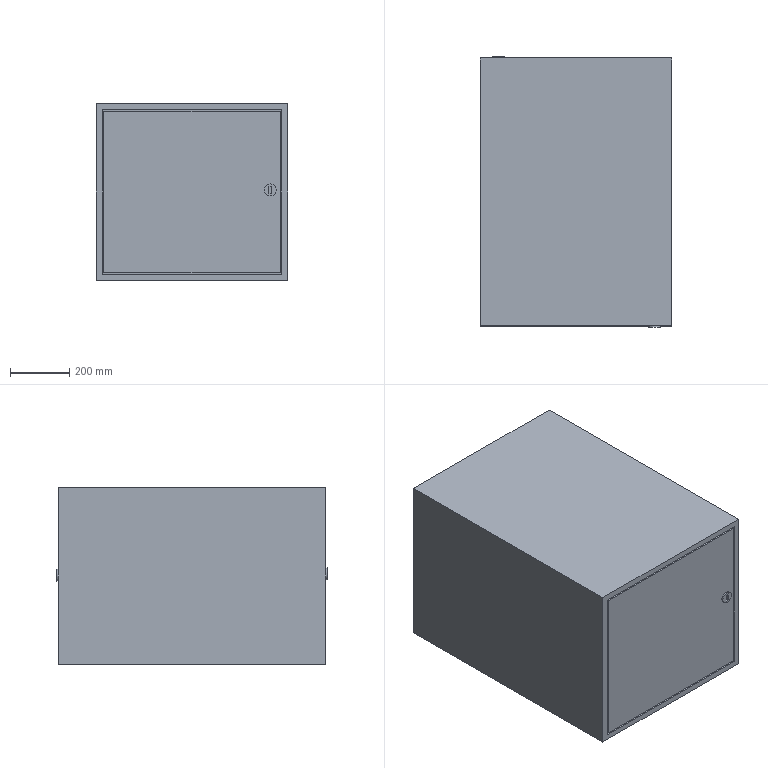Part | SolidWorks | features ICE 6, Extrusion 1 | 1 solid | 42 faces | box 645 x 910 x 594.5 mm | volume 344886947 mm3 | plane 38 | cylinder 4 | commonest cylinder face diameters 40 x4
STEP:
#1=CARTESIAN_POINT('',(-261.326,455.,320.206));
#2=VERTEX_POINT('',#1);
#3=CARTESIAN_POINT('',(-261.326,455.,280.206));
#4=VERTEX_POINT('',#3);
#5=CARTESIAN_POINT('',(-261.326,455.,300.206));
#6=DIRECTION('',(0.,1.,0.));
#7=DIRECTION('',(0.,0.,1.));
#8=AXIS2_PLACEMENT_3D('',#5,#6,#7);
#9=CIRCLE('',#8,20.);
#10=EDGE_CURVE('',#2,#4,#9,.T.);
#11=ORIENTED_EDGE('',*,*,#10,.F.);
#12=CARTESIAN_POINT('',(-261.326,450.,320.206));
#13=VERTEX_POINT('',#12);
#14=CARTESIAN_POINT('',(-261.326,455.,320.206));
#15=DIRECTION('',(0.,-1.,0.));
#16=VECTOR('',#15,1000.);
#17=LINE('',#14,#16);
#18=EDGE_CURVE('',#2,#13,#17,.T.);
#19=ORIENTED_EDGE('',*,*,#18,.T.);
#20=CARTESIAN_POINT('',(-261.326,450.,280.206));
#21=VERTEX_POINT('',#20);
#22=CARTESIAN_POINT('',(-261.326,450.,300.206));
#23=DIRECTION('',(0.,1.,0.));
#24=DIRECTION('',(0.,0.,-1.));
#25=AXIS2_PLACEMENT_3D('',#22,#23,#24);
#26=CIRCLE('',#25,20.);
#27=EDGE_CURVE('',#13,#21,#26,.T.);
#28=ORIENTED_EDGE('',*,*,#27,.T.);
#29=CARTESIAN_POINT('',(-261.326,455.,280.206));
#30=DIRECTION('',(0.,-1.,0.));
#31=VECTOR('',#30,1000.);
#32=LINE('',#29,#31);
#33=EDGE_CURVE('',#4,#21,#32,.T.);
#34=ORIENTED_EDGE('',*,*,#33,.F.);
#35=EDGE_LOOP('',(#11,#19,#28,#34));
#36=FACE_OUTER_BOUND('',#35,.T.);
#37=CARTESIAN_POINT('',(-261.326,455.,300.206));
#38=DIRECTION('',(0.,-1.,0.));
#39=DIRECTION('',(0.,0.,-1.));
#40=AXIS2_PLACEMENT_3D('',#37,#38,#39);
#41=CYLINDRICAL_SURFACE('',#40,20.);
#42=ADVANCED_FACE('',(#36),#41,.T.);
#43=CARTESIAN_POINT('',(263.592,-455.,284.23));
#44=VERTEX_POINT('',#43);
#45=CARTESIAN_POINT('',(263.592,-455.,324.23));
#46=VERTEX_POINT('',#45);
#47=CARTESIAN_POINT('',(263.592,-455.,304.23));
#48=DIRECTION('',(0.,-1.,0.));
#49=DIRECTION('',(0.,0.,-1.));
#50=AXIS2_PLACEMENT_3D('',#47,#48,#49);
#51=CIRCLE('',#50,20.);
#52=EDGE_CURVE('',#44,#46,#51,.T.);
#53=ORIENTED_EDGE('',*,*,#52,.F.);
#54=CARTESIAN_POINT('',(263.592,-450.,284.23));
#55=VERTEX_POINT('',#54);
#56=CARTESIAN_POINT('',(263.592,-455.,284.23));
#57=DIRECTION('',(0.,1.,0.));
#58=VECTOR('',#57,1000.);
#59=LINE('',#56,#58);
#60=EDGE_CURVE('',#44,#55,#59,.T.);
#61=ORIENTED_EDGE('',*,*,#60,.T.);
#62=CARTESIAN_POINT('',(263.592,-450.,324.23));
#63=VERTEX_POINT('',#62);
#64=CARTESIAN_POINT('',(263.592,-450.,304.23));
#65=DIRECTION('',(0.,-1.,0.));
#66=DIRECTION('',(0.,0.,1.));
#67=AXIS2_PLACEMENT_3D('',#64,#65,#66);
#68=CIRCLE('',#67,20.);
#69=EDGE_CURVE('',#55,#63,#68,.T.);
#70=ORIENTED_EDGE('',*,*,#69,.T.);
#71=CARTESIAN_POINT('',(263.592,-455.,324.23));
#72=DIRECTION('',(0.,1.,0.));
#73=VECTOR('',#72,1000.);
#74=LINE('',#71,#73);
#75=EDGE_CURVE('',#46,#63,#74,.T.);
#76=ORIENTED_EDGE('',*,*,#75,.F.);
#77=EDGE_LOOP('',(#53,#61,#70,#76));
#78=FACE_OUTER_BOUND('',#77,.T.);
#79=CARTESIAN_POINT('',(263.592,-455.,304.23));
#80=DIRECTION('',(0.,1.,0.));
#81=DIRECTION('',(0.,0.,1.));
#82=AXIS2_PLACEMENT_3D('',#79,#80,#81);
#83=CYLINDRICAL_SURFACE('',#82,20.);
#84=ADVANCED_FACE('',(#78),#83,.T.);
#85=CARTESIAN_POINT('',(322.5,-450.,0.));
#86=VERTEX_POINT('',#85);
#87=CARTESIAN_POINT('',(322.5,450.,0.));
#88=VERTEX_POINT('',#87);
#89=CARTESIAN_POINT('',(322.5,450.,0.));
#90=DIRECTION('',(0.,1.,0.));
#91=VECTOR('',#90,1000.);
#92=LINE('',#89,#91);
#93=EDGE_CURVE('',#86,#88,#92,.T.);
#94=ORIENTED_EDGE('',*,*,#93,.T.);
#95=CARTESIAN_POINT('',(322.5,450.,594.5));
#96=VERTEX_POINT('',#95);
#97=CARTESIAN_POINT('',(322.5,450.,594.5));
#98=DIRECTION('',(0.,0.,-1.));
#99=VECTOR('',#98,1000.);
#100=LINE('',#97,#99);
#101=EDGE_CURVE('',#96,#88,#100,.T.);
#102=ORIENTED_EDGE('',*,*,#101,.F.);
#103=CARTESIAN_POINT('',(322.5,-450.,594.5));
#104=VERTEX_POINT('',#103);
#105=CARTESIAN_POINT('',(322.5,450.,594.5));
#106=DIRECTION('',(0.,1.,0.));
#107=VECTOR('',#106,1000.);
#108=LINE('',#105,#107);
#109=EDGE_CURVE('',#104,#96,#108,.T.);
#110=ORIENTED_EDGE('',*,*,#109,.F.);
#111=CARTESIAN_POINT('',(322.5,-450.,594.5));
#112=DIRECTION('',(0.,0.,-1.));
#113=VECTOR('',#112,1000.);
#114=LINE('',#111,#113);
#115=EDGE_CURVE('',#104,#86,#114,.T.);
#116=ORIENTED_EDGE('',*,*,#115,.T.);
#117=EDGE_LOOP('',(#94,#102,#110,#116));
#118=FACE_OUTER_BOUND('',#117,.T.);
#119=CARTESIAN_POINT('',(322.5,450.,594.5));
#120=DIRECTION('',(-1.,0.,0.));
#121=DIRECTION('',(0.,-1.,0.));
#122=AXIS2_PLACEMENT_3D('',#119,#120,#121);
#123=PLANE('',#122);
#124=ADVANCED_FACE('',(#118),#123,.F.);
#125=CARTESIAN_POINT('',(-302.5,450.,574.5));
#126=VERTEX_POINT('',#125);
#127=CARTESIAN_POINT('',(302.5,450.,574.5));
#128=VERTEX_POINT('',#127);
#129=CARTESIAN_POINT('',(-302.5,450.,574.5));
#130=DIRECTION('',(1.,0.,0.));
#131=VECTOR('',#130,1000.);
#132=LINE('',#129,#131);
#133=EDGE_CURVE('',#126,#128,#132,.T.);
#134=ORIENTED_EDGE('',*,*,#133,.F.);
#135=CARTESIAN_POINT('',(-302.5,450.,20.));
#136=VERTEX_POINT('',#135);
#137=CARTESIAN_POINT('',(-302.5,450.,20.));
#138=DIRECTION('',(0.,0.,1.));
#139=VECTOR('',#138,1000.);
#140=LINE('',#137,#139);
#141=EDGE_CURVE('',#136,#126,#140,.T.);
#142=ORIENTED_EDGE('',*,*,#141,.F.);
#143=CARTESIAN_POINT('',(302.5,450.,20.));
#144=VERTEX_POINT('',#143);
#145=CARTESIAN_POINT('',(302.5,450.,20.));
#146=DIRECTION('',(-1.,0.,0.));
#147=VECTOR('',#146,1000.);
#148=LINE('',#145,#147);
#149=EDGE_CURVE('',#144,#136,#148,.T.);
#150=ORIENTED_EDGE('',*,*,#149,.F.);
#151=CARTESIAN_POINT('',(302.5,450.,574.5));
#152=DIRECTION('',(0.,0.,-1.));
#153=VECTOR('',#152,1000.);
#154=LINE('',#151,#153);
#155=EDGE_CURVE('',#128,#144,#154,.T.);
#156=ORIENTED_EDGE('',*,*,#155,.F.);
#157=EDGE_LOOP('',(#134,#142,#150,#156));
#158=FACE_BOUND('',#157,.T.);
#159=CARTESIAN_POINT('',(-322.5,450.,0.));
#160=VERTEX_POINT('',#159);
#161=CARTESIAN_POINT('',(-322.5,450.,0.));
#162=DIRECTION('',(-1.,0.,0.));
#163=VECTOR('',#162,1000.);
#164=LINE('',#161,#163);
#165=EDGE_CURVE('',#88,#160,#164,.T.);
#166=ORIENTED_EDGE('',*,*,#165,.T.);
#167=CARTESIAN_POINT('',(-322.5,450.,594.5));
#168=VERTEX_POINT('',#167);
#169=CARTESIAN_POINT('',(-322.5,450.,594.5));
#170=DIRECTION('',(0.,0.,-1.));
#171=VECTOR('',#170,1000.);
#172=LINE('',#169,#171);
#173=EDGE_CURVE('',#168,#160,#172,.T.);
#174=ORIENTED_EDGE('',*,*,#173,.F.);
#175=CARTESIAN_POINT('',(-322.5,450.,594.5));
#176=DIRECTION('',(-1.,0.,0.));
#177=VECTOR('',#176,1000.);
#178=LINE('',#175,#177);
#179=EDGE_CURVE('',#96,#168,#178,.T.);
#180=ORIENTED_EDGE('',*,*,#179,.F.);
#181=ORIENTED_EDGE('',*,*,#101,.T.);
#182=EDGE_LOOP('',(#166,#174,#180,#181));
#183=FACE_OUTER_BOUND('',#182,.T.);
#184=CARTESIAN_POINT('',(-322.5,450.,594.5));
#185=DIRECTION('',(0.,-1.,0.));
#186=DIRECTION('',(0.,0.,-1.));
#187=AXIS2_PLACEMENT_3D('',#184,#185,#186);
#188=PLANE('',#187);
#189=ADVANCED_FACE('',(#158,#183),#188,.F.);
#190=CARTESIAN_POINT('',(-322.5,-450.,0.));
#191=VERTEX_POINT('',#190);
#192=CARTESIAN_POINT('',(-322.5,450.,0.));
#193=DIRECTION('',(0.,-1.,0.));
#194=VECTOR('',#193,1000.);
#195=LINE('',#192,#194);
#196=EDGE_CURVE('',#160,#191,#195,.T.);
#197=ORIENTED_EDGE('',*,*,#196,.T.);
#198=CARTESIAN_POINT('',(-322.5,-450.,594.5));
#199=VERTEX_POINT('',#198);
#200=CARTESIAN_POINT('',(-322.5,-450.,594.5));
#201=DIRECTION('',(0.,0.,-1.));
#202=VECTOR('',#201,1000.);
#203=LINE('',#200,#202);
#204=EDGE_CURVE('',#199,#191,#203,.T.);
#205=ORIENTED_EDGE('',*,*,#204,.F.);
#206=CARTESIAN_POINT('',(-322.5,450.,594.5));
#207=DIRECTION('',(0.,-1.,0.));
#208=VECTOR('',#207,1000.);
#209=LINE('',#206,#208);
#210=EDGE_CURVE('',#168,#199,#209,.T.);
#211=ORIENTED_EDGE('',*,*,#210,.F.);
#212=ORIENTED_EDGE('',*,*,#173,.T.);
#213=EDGE_LOOP('',(#197,#205,#211,#212));
#214=FACE_OUTER_BOUND('',#213,.T.);
#215=CARTESIAN_POINT('',(-322.5,450.,594.5));
#216=DIRECTION('',(1.,0.,0.));
#217=DIRECTION('',(0.,1.,0.));
#218=AXIS2_PLACEMENT_3D('',#215,#216,#217);
#219=PLANE('',#218);
#220=ADVANCED_FACE('',(#214),#219,.F.);
#221=CARTESIAN_POINT('',(302.5,-450.,574.5));
#222=VERTEX_POINT('',#221);
#223=CARTESIAN_POINT('',(-302.5,-450.,574.5));
#224=VERTEX_POINT('',#223);
#225=CARTESIAN_POINT('',(-302.5,-450.,574.5));
#226=DIRECTION('',(-1.,0.,0.));
#227=VECTOR('',#226,1000.);
#228=LINE('',#225,#227);
#229=EDGE_CURVE('',#222,#224,#228,.T.);
#230=ORIENTED_EDGE('',*,*,#229,.F.);
#231=CARTESIAN_POINT('',(302.5,-450.,20.));
#232=VERTEX_POINT('',#231);
#233=CARTESIAN_POINT('',(302.5,-450.,574.5));
#234=DIRECTION('',(0.,0.,1.));
#235=VECTOR('',#234,1000.);
#236=LINE('',#233,#235);
#237=EDGE_CURVE('',#232,#222,#236,.T.);
#238=ORIENTED_EDGE('',*,*,#237,.F.);
#239=CARTESIAN_POINT('',(-302.5,-450.,20.));
#240=VERTEX_POINT('',#239);
#241=CARTESIAN_POINT('',(-302.5,-450.,20.));
#242=DIRECTION('',(1.,0.,0.));
#243=VECTOR('',#242,1000.);
#244=LINE('',#241,#243);
#245=EDGE_CURVE('',#240,#232,#244,.T.);
#246=ORIENTED_EDGE('',*,*,#245,.F.);
#247=CARTESIAN_POINT('',(-302.5,-450.,574.5));
#248=DIRECTION('',(0.,0.,-1.));
#249=VECTOR('',#248,1000.);
#250=LINE('',#247,#249);
#251=EDGE_CURVE('',#224,#240,#250,.T.);
#252=ORIENTED_EDGE('',*,*,#251,.F.);
#253=EDGE_LOOP('',(#230,#238,#246,#252));
#254=FACE_BOUND('',#253,.T.);
#255=CARTESIAN_POINT('',(-322.5,-450.,0.));
#256=DIRECTION('',(1.,0.,0.));
#257=VECTOR('',#256,1000.);
#258=LINE('',#255,#257);
#259=EDGE_CURVE('',#191,#86,#258,.T.);
#260=ORIENTED_EDGE('',*,*,#259,.T.);
#261=ORIENTED_EDGE('',*,*,#115,.F.);
#262=CARTESIAN_POINT('',(-322.5,-450.,594.5));
#263=DIRECTION('',(1.,0.,0.));
#264=VECTOR('',#263,1000.);
#265=LINE('',#262,#264);
#266=EDGE_CURVE('',#199,#104,#265,.T.);
#267=ORIENTED_EDGE('',*,*,#266,.F.);
#268=ORIENTED_EDGE('',*,*,#204,.T.);
#269=EDGE_LOOP('',(#260,#261,#267,#268));
#270=FACE_OUTER_BOUND('',#269,.T.);
#271=CARTESIAN_POINT('',(-322.5,-450.,594.5));
#272=DIRECTION('',(0.,1.,0.));
#273=DIRECTION('',(0.,0.,1.));
#274=AXIS2_PLACEMENT_3D('',#271,#272,#273);
#275=PLANE('',#274);
#276=ADVANCED_FACE('',(#254,#270),#275,.F.);
#277=ORIENTED_EDGE('',*,*,#109,.T.);
#278=ORIENTED_EDGE('',*,*,#179,.T.);
#279=ORIENTED_EDGE('',*,*,#210,.T.);
#280=ORIENTED_EDGE('',*,*,#266,.T.);
#281=EDGE_LOOP('',(#277,#278,#279,#280));
#282=FACE_OUTER_BOUND('',#281,.T.);
#283=CARTESIAN_POINT('',(0.,0.,594.5));
#284=DIRECTION('',(0.,0.,1.));
#285=DIRECTION('',(1.,0.,0.));
#286=AXIS2_PLACEMENT_3D('',#283,#284,#285);
#287=PLANE('',#286);
#288=ADVANCED_FACE('',(#282),#287,.T.);
#289=ORIENTED_EDGE('',*,*,#93,.F.);
#290=ORIENTED_EDGE('',*,*,#259,.F.);
#291=ORIENTED_EDGE('',*,*,#196,.F.);
#292=ORIENTED_EDGE('',*,*,#165,.F.);
#293=EDGE_LOOP('',(#289,#290,#291,#292));
#294=FACE_OUTER_BOUND('',#293,.T.);
#295=CARTESIAN_POINT('',(0.,0.,0.));
#296=DIRECTION('',(0.,0.,1.));
#297=DIRECTION('',(1.,0.,0.));
#298=AXIS2_PLACEMENT_3D('',#295,#296,#297);
#299=PLANE('',#298);
#300=ADVANCED_FACE('',(#294),#299,.F.);
#301=ORIENTED_EDGE('',*,*,#237,.T.);
#302=CARTESIAN_POINT('',(302.5,-440.,574.5));
#303=VERTEX_POINT('',#302);
#304=CARTESIAN_POINT('',(302.5,-440.,574.5));
#305=DIRECTION('',(0.,-1.,0.));
#306=VECTOR('',#305,1000.);
#307=LINE('',#304,#306);
#308=EDGE_CURVE('',#303,#222,#307,.T.);
#309=ORIENTED_EDGE('',*,*,#308,.F.);
#310=CARTESIAN_POINT('',(302.5,-440.,20.));
#311=VERTEX_POINT('',#310);
#312=CARTESIAN_POINT('',(302.5,-440.,574.5));
#313=DIRECTION('',(0.,0.,1.));
#314=VECTOR('',#313,1000.);
#315=LINE('',#312,#314);
#316=EDGE_CURVE('',#311,#303,#315,.T.);
#317=ORIENTED_EDGE('',*,*,#316,.F.);
#318=CARTESIAN_POINT('',(302.5,-440.,20.));
#319=DIRECTION('',(0.,-1.,0.));
#320=VECTOR('',#319,1000.);
#321=LINE('',#318,#320);
#322=EDGE_CURVE('',#311,#232,#321,.T.);
#323=ORIENTED_EDGE('',*,*,#322,.T.);
#324=EDGE_LOOP('',(#301,#309,#317,#323));
#325=FACE_OUTER_BOUND('',#324,.T.);
#326=CARTESIAN_POINT('',(302.5,-440.,574.5));
#327=DIRECTION('',(1.,0.,0.));
#328=DIRECTION('',(0.,0.,-1.));
#329=AXIS2_PLACEMENT_3D('',#326,#327,#328);
#330=PLANE('',#329);
#331=ADVANCED_FACE('',(#325),#330,.F.);
#332=ORIENTED_EDGE('',*,*,#245,.T.);
#333=ORIENTED_EDGE('',*,*,#322,.F.);
#334=CARTESIAN_POINT('',(-302.5,-440.,20.));
#335=VERTEX_POINT('',#334);
#336=CARTESIAN_POINT('',(-302.5,-440.,20.));
#337=DIRECTION('',(1.,0.,0.));
#338=VECTOR('',#337,1000.);
#339=LINE('',#336,#338);
#340=EDGE_CURVE('',#335,#311,#339,.T.);
#341=ORIENTED_EDGE('',*,*,#340,.F.);
#342=CARTESIAN_POINT('',(-302.5,-440.,20.));
#343=DIRECTION('',(0.,-1.,0.));
#344=VECTOR('',#343,1000.);
#345=LINE('',#342,#344);
#346=EDGE_CURVE('',#335,#240,#345,.T.);
#347=ORIENTED_EDGE('',*,*,#346,.T.);
#348=EDGE_LOOP('',(#332,#333,#341,#347));
#349=FACE_OUTER_BOUND('',#348,.T.);
#350=CARTESIAN_POINT('',(-302.5,-440.,20.));
#351=DIRECTION('',(0.,0.,-1.));
#352=DIRECTION('',(-1.,0.,0.));
#353=AXIS2_PLACEMENT_3D('',#350,#351,#352);
#354=PLANE('',#353);
#355=ADVANCED_FACE('',(#349),#354,.F.);
#356=ORIENTED_EDGE('',*,*,#251,.T.);
#357=ORIENTED_EDGE('',*,*,#346,.F.);
#358=CARTESIAN_POINT('',(-302.5,-440.,574.5));
#359=VERTEX_POINT('',#358);
#360=CARTESIAN_POINT('',(-302.5,-440.,574.5));
#361=DIRECTION('',(0.,0.,-1.));
#362=VECTOR('',#361,1000.);
#363=LINE('',#360,#362);
#364=EDGE_CURVE('',#359,#335,#363,.T.);
#365=ORIENTED_EDGE('',*,*,#364,.F.);
#366=CARTESIAN_POINT('',(-302.5,-440.,574.5));
#367=DIRECTION('',(0.,-1.,0.));
#368=VECTOR('',#367,1000.);
#369=LINE('',#366,#368);
#370=EDGE_CURVE('',#359,#224,#369,.T.);
#371=ORIENTED_EDGE('',*,*,#370,.T.);
#372=EDGE_LOOP('',(#356,#357,#365,#371));
#373=FACE_OUTER_BOUND('',#372,.T.);
#374=CARTESIAN_POINT('',(-302.5,-440.,574.5));
#375=DIRECTION('',(-1.,0.,0.));
#376=DIRECTION('',(0.,0.,1.));
#377=AXIS2_PLACEMENT_3D('',#374,#375,#376);
#378=PLANE('',#377);
#379=ADVANCED_FACE('',(#373),#378,.F.);
#380=ORIENTED_EDGE('',*,*,#229,.T.);
#381=ORIENTED_EDGE('',*,*,#370,.F.);
#382=CARTESIAN_POINT('',(-302.5,-440.,574.5));
#383=DIRECTION('',(-1.,0.,0.));
#384=VECTOR('',#383,1000.);
#385=LINE('',#382,#384);
#386=EDGE_CURVE('',#303,#359,#385,.T.);
#387=ORIENTED_EDGE('',*,*,#386,.F.);
#388=ORIENTED_EDGE('',*,*,#308,.T.);
#389=EDGE_LOOP('',(#380,#381,#387,#388));
#390=FACE_OUTER_BOUND('',#389,.T.);
#391=CARTESIAN_POINT('',(-302.5,-440.,574.5));
#392=DIRECTION('',(0.,0.,1.));
#393=DIRECTION('',(1.,0.,0.));
#394=AXIS2_PLACEMENT_3D('',#391,#392,#393);
#395=PLANE('',#394);
#396=ADVANCED_FACE('',(#390),#395,.F.);
#397=CARTESIAN_POINT('',(297.5,-440.,569.5));
#398=VERTEX_POINT('',#397);
#399=CARTESIAN_POINT('',(-297.5,-440.,569.5));
#400=VERTEX_POINT('',#399);
#401=CARTESIAN_POINT('',(-297.5,-440.,569.5));
#402=DIRECTION('',(-1.,0.,0.));
#403=VECTOR('',#402,1000.);
#404=LINE('',#401,#403);
#405=EDGE_CURVE('',#398,#400,#404,.T.);
#406=ORIENTED_EDGE('',*,*,#405,.F.);
#407=CARTESIAN_POINT('',(297.5,-440.,25.));
#408=VERTEX_POINT('',#407);
#409=CARTESIAN_POINT('',(297.5,-440.,569.5));
#410=DIRECTION('',(0.,0.,1.));
#411=VECTOR('',#410,1000.);
#412=LINE('',#409,#411);
#413=EDGE_CURVE('',#408,#398,#412,.T.);
#414=ORIENTED_EDGE('',*,*,#413,.F.);
#415=CARTESIAN_POINT('',(-297.5,-440.,25.));
#416=VERTEX_POINT('',#415);
#417=CARTESIAN_POINT('',(-297.5,-440.,25.));
#418=DIRECTION('',(1.,0.,0.));
#419=VECTOR('',#418,1000.);
#420=LINE('',#417,#419);
#421=EDGE_CURVE('',#416,#408,#420,.T.);
#422=ORIENTED_EDGE('',*,*,#421,.F.);
#423=CARTESIAN_POINT('',(-297.5,-440.,569.5));
#424=DIRECTION('',(0.,0.,-1.));
#425=VECTOR('',#424,1000.);
#426=LINE('',#423,#425);
#427=EDGE_CURVE('',#400,#416,#426,.T.);
#428=ORIENTED_EDGE('',*,*,#427,.F.);
#429=EDGE_LOOP('',(#406,#414,#422,#428));
#430=FACE_BOUND('',#429,.T.);
#431=ORIENTED_EDGE('',*,*,#316,.T.);
#432=ORIENTED_EDGE('',*,*,#386,.T.);
#433=ORIENTED_EDGE('',*,*,#364,.T.);
#434=ORIENTED_EDGE('',*,*,#340,.T.);
#435=EDGE_LOOP('',(#431,#432,#433,#434));
#436=FACE_OUTER_BOUND('',#435,.T.);
#437=CARTESIAN_POINT('',(0.,-440.,0.));
#438=DIRECTION('',(0.,-1.,0.));
#439=DIRECTION('',(0.,0.,-1.));
#440=AXIS2_PLACEMENT_3D('',#437,#438,#439);
#441=PLANE('',#440);
#442=ADVANCED_FACE('',(#430,#436),#441,.T.);
#443=CARTESIAN_POINT('',(-297.5,-450.,569.5));
#444=VERTEX_POINT('',#443);
#445=CARTESIAN_POINT('',(-297.5,-450.,25.));
#446=VERTEX_POINT('',#445);
#447=CARTESIAN_POINT('',(-297.5,-450.,569.5));
#448=DIRECTION('',(0.,0.,-1.));
#449=VECTOR('',#448,1000.);
#450=LINE('',#447,#449);
#451=EDGE_CURVE('',#444,#446,#450,.T.);
#452=ORIENTED_EDGE('',*,*,#451,.F.);
#453=CARTESIAN_POINT('',(-297.5,-440.,569.5));
#454=DIRECTION('',(0.,-1.,0.));
#455=VECTOR('',#454,1000.);
#456=LINE('',#453,#455);
#457=EDGE_CURVE('',#400,#444,#456,.T.);
#458=ORIENTED_EDGE('',*,*,#457,.F.);
#459=ORIENTED_EDGE('',*,*,#427,.T.);
#460=CARTESIAN_POINT('',(-297.5,-440.,25.));
#461=DIRECTION('',(0.,-1.,0.));
#462=VECTOR('',#461,1000.);
#463=LINE('',#460,#462);
#464=EDGE_CURVE('',#416,#446,#463,.T.);
#465=ORIENTED_EDGE('',*,*,#464,.T.);
#466=EDGE_LOOP('',(#452,#458,#459,#465));
#467=FACE_OUTER_BOUND('',#466,.T.);
#468=CARTESIAN_POINT('',(-297.5,-440.,569.5));
#469=DIRECTION('',(-1.,0.,0.));
#470=DIRECTION('',(0.,0.,1.));
#471=AXIS2_PLACEMENT_3D('',#468,#469,#470);
#472=PLANE('',#471);
#473=ADVANCED_FACE('',(#467),#472,.T.);
#474=CARTESIAN_POINT('',(297.5,-450.,569.5));
#475=VERTEX_POINT('',#474);
#476=CARTESIAN_POINT('',(-297.5,-450.,569.5));
#477=DIRECTION('',(-1.,0.,0.));
#478=VECTOR('',#477,1000.);
#479=LINE('',#476,#478);
#480=EDGE_CURVE('',#475,#444,#479,.T.);
#481=ORIENTED_EDGE('',*,*,#480,.F.);
#482=CARTESIAN_POINT('',(297.5,-440.,569.5));
#483=DIRECTION('',(0.,-1.,0.));
#484=VECTOR('',#483,1000.);
#485=LINE('',#482,#484);
#486=EDGE_CURVE('',#398,#475,#485,.T.);
#487=ORIENTED_EDGE('',*,*,#486,.F.);
#488=ORIENTED_EDGE('',*,*,#405,.T.);
#489=ORIENTED_EDGE('',*,*,#457,.T.);
#490=EDGE_LOOP('',(#481,#487,#488,#489));
#491=FACE_OUTER_BOUND('',#490,.T.);
#492=CARTESIAN_POINT('',(-297.5,-440.,569.5));
#493=DIRECTION('',(0.,0.,1.));
#494=DIRECTION('',(1.,0.,0.));
#495=AXIS2_PLACEMENT_3D('',#492,#493,#494);
#496=PLANE('',#495);
#497=ADVANCED_FACE('',(#491),#496,.T.);
#498=CARTESIAN_POINT('',(297.5,-450.,25.));
#499=VERTEX_POINT('',#498);
#500=CARTESIAN_POINT('',(297.5,-450.,569.5));
#501=DIRECTION('',(0.,0.,1.));
#502=VECTOR('',#501,1000.);
#503=LINE('',#500,#502);
#504=EDGE_CURVE('',#499,#475,#503,.T.);
#505=ORIENTED_EDGE('',*,*,#504,.F.);
#506=CARTESIAN_POINT('',(297.5,-440.,25.));
#507=DIRECTION('',(0.,-1.,0.));
#508=VECTOR('',#507,1000.);
#509=LINE('',#506,#508);
#510=EDGE_CURVE('',#408,#499,#509,.T.);
#511=ORIENTED_EDGE('',*,*,#510,.F.);
#512=ORIENTED_EDGE('',*,*,#413,.T.);
#513=ORIENTED_EDGE('',*,*,#486,.T.);
#514=EDGE_LOOP('',(#505,#511,#512,#513));
#515=FACE_OUTER_BOUND('',#514,.T.);
#516=CARTESIAN_POINT('',(297.5,-440.,569.5));
#517=DIRECTION('',(1.,0.,0.));
#518=DIRECTION('',(0.,0.,-1.));
#519=AXIS2_PLACEMENT_3D('',#516,#517,#518);
#520=PLANE('',#519);
#521=ADVANCED_FACE('',(#515),#520,.T.);
#522=CARTESIAN_POINT('',(-297.5,-450.,25.));
#523=DIRECTION('',(1.,0.,0.));
#524=VECTOR('',#523,1000.);
#525=LINE('',#522,#524);
#526=EDGE_CURVE('',#446,#499,#525,.T.);
#527=ORIENTED_EDGE('',*,*,#526,.F.);
#528=ORIENTED_EDGE('',*,*,#464,.F.);
#529=ORIENTED_EDGE('',*,*,#421,.T.);
#530=ORIENTED_EDGE('',*,*,#510,.T.);
#531=EDGE_LOOP('',(#527,#528,#529,#530));
#532=FACE_OUTER_BOUND('',#531,.T.);
#533=CARTESIAN_POINT('',(-297.5,-440.,25.));
#534=DIRECTION('',(0.,0.,-1.));
#535=DIRECTION('',(-1.,0.,0.));
#536=AXIS2_PLACEMENT_3D('',#533,#534,#535);
#537=PLANE('',#536);
#538=ADVANCED_FACE('',(#532),#537,.T.);
#539=CARTESIAN_POINT('',(263.592,-450.,304.23));
#540=DIRECTION('',(0.,-1.,0.));
#541=DIRECTION('',(0.,0.,1.));
#542=AXIS2_PLACEMENT_3D('',#539,#540,#541);
#543=CIRCLE('',#542,20.);
#544=EDGE_CURVE('',#63,#55,#543,.T.);
#545=ORIENTED_EDGE('',*,*,#544,.F.);
#546=ORIENTED_EDGE('',*,*,#69,.F.);
#547=EDGE_LOOP('',(#545,#546));
#548=FACE_BOUND('',#547,.T.);
#549=ORIENTED_EDGE('',*,*,#451,.T.);
#550=ORIENTED_EDGE('',*,*,#526,.T.);
#551=ORIENTED_EDGE('',*,*,#504,.T.);
#552=ORIENTED_EDGE('',*,*,#480,.T.);
#553=EDGE_LOOP('',(#549,#550,#551,#552));
#554=FACE_OUTER_BOUND('',#553,.T.);
#555=CARTESIAN_POINT('',(-322.5,-450.,594.5));
#556=DIRECTION('',(0.,1.,0.));
#557=DIRECTION('',(0.,0.,1.));
#558=AXIS2_PLACEMENT_3D('',#555,#556,#557);
#559=PLANE('',#558);
#560=ADVANCED_FACE('',(#548,#554),#559,.F.);
#561=ORIENTED_EDGE('',*,*,#60,.F.);
#562=CARTESIAN_POINT('',(263.592,-455.,304.23));
#563=DIRECTION('',(0.,-1.,0.));
#564=DIRECTION('',(0.,0.,-1.));
#565=AXIS2_PLACEMENT_3D('',#562,#563,#564);
#566=CIRCLE('',#565,20.);
#567=EDGE_CURVE('',#46,#44,#566,.T.);
#568=ORIENTED_EDGE('',*,*,#567,.F.);
#569=ORIENTED_EDGE('',*,*,#75,.T.);
#570=ORIENTED_EDGE('',*,*,#544,.T.);
#571=EDGE_LOOP('',(#561,#568,#569,#570));
#572=FACE_OUTER_BOUND('',#571,.T.);
#573=CARTESIAN_POINT('',(263.592,-455.,304.23));
#574=DIRECTION('',(0.,1.,0.));
#575=DIRECTION('',(0.,0.,1.));
#576=AXIS2_PLACEMENT_3D('',#573,#574,#575);
#577=CYLINDRICAL_SURFACE('',#576,20.);
#578=ADVANCED_FACE('',(#572),#577,.T.);
#579=CARTESIAN_POINT('',(258.627,-455.,316.56));
#580=VERTEX_POINT('',#579);
#581=CARTESIAN_POINT('',(258.627,-455.,291.9));
#582=VERTEX_POINT('',#581);
#583=CARTESIAN_POINT('',(258.627,-455.,316.56));
#584=DIRECTION('',(0.,0.,-1.));
#585=VECTOR('',#584,1000.);
#586=LINE('',#583,#585);
#587=EDGE_CURVE('',#580,#582,#586,.T.);
#588=ORIENTED_EDGE('',*,*,#587,.F.);
#589=CARTESIAN_POINT('',(268.558,-455.,316.56));
#590=VERTEX_POINT('',#589);
#591=CARTESIAN_POINT('',(268.558,-455.,316.56));
#592=DIRECTION('',(-1.,0.,0.));
#593=VECTOR('',#592,1000.);
#594=LINE('',#591,#593);
#595=EDGE_CURVE('',#590,#580,#594,.T.);
#596=ORIENTED_EDGE('',*,*,#595,.F.);
#597=CARTESIAN_POINT('',(268.558,-455.,291.9));
#598=VERTEX_POINT('',#597);
#599=CARTESIAN_POINT('',(268.558,-455.,316.56));
#600=DIRECTION('',(0.,0.,1.));
#601=VECTOR('',#600,1000.);
#602=LINE('',#599,#601);
#603=EDGE_CURVE('',#598,#590,#602,.T.);
#604=ORIENTED_EDGE('',*,*,#603,.F.);
#605=CARTESIAN_POINT('',(268.558,-455.,291.9));
#606=DIRECTION('',(1.,0.,0.));
#607=VECTOR('',#606,1000.);
#608=LINE('',#605,#607);
#609=EDGE_CURVE('',#582,#598,#608,.T.);
#610=ORIENTED_EDGE('',*,*,#609,.F.);
#611=EDGE_LOOP('',(#588,#596,#604,#610));
#612=FACE_BOUND('',#611,.T.);
#613=ORIENTED_EDGE('',*,*,#567,.T.);
#614=ORIENTED_EDGE('',*,*,#52,.T.);
#615=EDGE_LOOP('',(#613,#614));
#616=FACE_OUTER_BOUND('',#615,.T.);
#617=CARTESIAN_POINT('',(263.592,-455.,304.23));
#618=DIRECTION('',(0.,-1.,0.));
#619=DIRECTION('',(0.,0.,-1.));
#620=AXIS2_PLACEMENT_3D('',#617,#618,#619);
#621=PLANE('',#620);
#622=ADVANCED_FACE('',(#612,#616),#621,.T.);
#623=ORIENTED_EDGE('',*,*,#587,.T.);
#624=CARTESIAN_POINT('',(258.627,-450.,291.9));
#625=VERTEX_POINT('',#624);
#626=CARTESIAN_POINT('',(258.627,-450.,291.9));
#627=DIRECTION('',(0.,-1.,0.));
#628=VECTOR('',#627,1000.);
#629=LINE('',#626,#628);
#630=EDGE_CURVE('',#625,#582,#629,.T.);
#631=ORIENTED_EDGE('',*,*,#630,.F.);
#632=CARTESIAN_POINT('',(258.627,-450.,316.56));
#633=VERTEX_POINT('',#632);
#634=CARTESIAN_POINT('',(258.627,-450.,316.56));
#635=DIRECTION('',(0.,0.,-1.));
#636=VECTOR('',#635,1000.);
#637=LINE('',#634,#636);
#638=EDGE_CURVE('',#633,#625,#637,.T.);
#639=ORIENTED_EDGE('',*,*,#638,.F.);
#640=CARTESIAN_POINT('',(258.627,-450.,316.56));
#641=DIRECTION('',(0.,-1.,0.));
#642=VECTOR('',#641,1000.);
#643=LINE('',#640,#642);
#644=EDGE_CURVE('',#633,#580,#643,.T.);
#645=ORIENTED_EDGE('',*,*,#644,.T.);
#646=EDGE_LOOP('',(#623,#631,#639,#645));
#647=FACE_OUTER_BOUND('',#646,.T.);
#648=CARTESIAN_POINT('',(258.627,-450.,316.56));
#649=DIRECTION('',(-1.,0.,0.));
#650=DIRECTION('',(0.,0.,1.));
#651=AXIS2_PLACEMENT_3D('',#648,#649,#650);
#652=PLANE('',#651);
#653=ADVANCED_FACE('',(#647),#652,.F.);
#654=ORIENTED_EDGE('',*,*,#595,.T.);
#655=ORIENTED_EDGE('',*,*,#644,.F.);
#656=CARTESIAN_POINT('',(268.558,-450.,316.56));
#657=VERTEX_POINT('',#656);
#658=CARTESIAN_POINT('',(268.558,-450.,316.56));
#659=DIRECTION('',(-1.,0.,0.));
#660=VECTOR('',#659,1000.);
#661=LINE('',#658,#660);
#662=EDGE_CURVE('',#657,#633,#661,.T.);
#663=ORIENTED_EDGE('',*,*,#662,.F.);
#664=CARTESIAN_POINT('',(268.558,-450.,316.56));
#665=DIRECTION('',(0.,-1.,0.));
#666=VECTOR('',#665,1000.);
#667=LINE('',#664,#666);
#668=EDGE_CURVE('',#657,#590,#667,.T.);
#669=ORIENTED_EDGE('',*,*,#668,.T.);
#670=EDGE_LOOP('',(#654,#655,#663,#669));
#671=FACE_OUTER_BOUND('',#670,.T.);
#672=CARTESIAN_POINT('',(268.558,-450.,316.56));
#673=DIRECTION('',(0.,0.,1.));
#674=DIRECTION('',(1.,0.,0.));
#675=AXIS2_PLACEMENT_3D('',#672,#673,#674);
#676=PLANE('',#675);
#677=ADVANCED_FACE('',(#671),#676,.F.);
#678=ORIENTED_EDGE('',*,*,#603,.T.);
#679=ORIENTED_EDGE('',*,*,#668,.F.);
#680=CARTESIAN_POINT('',(268.558,-450.,291.9));
#681=VERTEX_POINT('',#680);
#682=CARTESIAN_POINT('',(268.558,-450.,316.56));
#683=DIRECTION('',(0.,0.,1.));
#684=VECTOR('',#683,1000.);
#685=LINE('',#682,#684);
#686=EDGE_CURVE('',#681,#657,#685,.T.);
#687=ORIENTED_EDGE('',*,*,#686,.F.);
#688=CARTESIAN_POINT('',(268.558,-450.,291.9));
#689=DIRECTION('',(0.,-1.,0.));
#690=VECTOR('',#689,1000.);
#691=LINE('',#688,#690);
#692=EDGE_CURVE('',#681,#598,#691,.T.);
#693=ORIENTED_EDGE('',*,*,#692,.T.);
#694=EDGE_LOOP('',(#678,#679,#687,#693));
#695=FACE_OUTER_BOUND('',#694,.T.);
#696=CARTESIAN_POINT('',(268.558,-450.,316.56));
#697=DIRECTION('',(1.,0.,0.));
#698=DIRECTION('',(0.,0.,-1.));
#699=AXIS2_PLACEMENT_3D('',#696,#697,#698);
#700=PLANE('',#699);
#701=ADVANCED_FACE('',(#695),#700,.F.);
#702=ORIENTED_EDGE('',*,*,#609,.T.);
#703=ORIENTED_EDGE('',*,*,#692,.F.);
#704=CARTESIAN_POINT('',(268.558,-450.,291.9));
#705=DIRECTION('',(1.,0.,0.));
#706=VECTOR('',#705,1000.);
#707=LINE('',#704,#706);
#708=EDGE_CURVE('',#625,#681,#707,.T.);
#709=ORIENTED_EDGE('',*,*,#708,.F.);
#710=ORIENTED_EDGE('',*,*,#630,.T.);
#711=EDGE_LOOP('',(#702,#703,#709,#710));
#712=FACE_OUTER_BOUND('',#711,.T.);
#713=CARTESIAN_POINT('',(268.558,-450.,291.9));
#714=DIRECTION('',(0.,0.,-1.));
#715=DIRECTION('',(-1.,0.,0.));
#716=AXIS2_PLACEMENT_3D('',#713,#714,#715);
#717=PLANE('',#716);
#718=ADVANCED_FACE('',(#712),#717,.F.);
#719=ORIENTED_EDGE('',*,*,#638,.T.);
#720=ORIENTED_EDGE('',*,*,#708,.T.);
#721=ORIENTED_EDGE('',*,*,#686,.T.);
#722=ORIENTED_EDGE('',*,*,#662,.T.);
#723=EDGE_LOOP('',(#719,#720,#721,#722));
#724=FACE_OUTER_BOUND('',#723,.T.);
#725=CARTESIAN_POINT('',(0.,-450.,0.));
#726=DIRECTION('',(0.,1.,0.));
#727=DIRECTION('',(0.,0.,1.));
#728=AXIS2_PLACEMENT_3D('',#725,#726,#727);
#729=PLANE('',#728);
#730=ADVANCED_FACE('',(#724),#729,.F.);
#731=ORIENTED_EDGE('',*,*,#141,.T.);
#732=CARTESIAN_POINT('',(-302.5,440.,574.5));
#733=VERTEX_POINT('',#732);
#734=CARTESIAN_POINT('',(-302.5,440.,574.5));
#735=DIRECTION('',(0.,1.,0.));
#736=VECTOR('',#735,1000.);
#737=LINE('',#734,#736);
#738=EDGE_CURVE('',#733,#126,#737,.T.);
#739=ORIENTED_EDGE('',*,*,#738,.F.);
#740=CARTESIAN_POINT('',(-302.5,440.,20.));
#741=VERTEX_POINT('',#740);
#742=CARTESIAN_POINT('',(-302.5,440.,20.));
#743=DIRECTION('',(0.,0.,1.));
#744=VECTOR('',#743,1000.);
#745=LINE('',#742,#744);
#746=EDGE_CURVE('',#741,#733,#745,.T.);
#747=ORIENTED_EDGE('',*,*,#746,.F.);
#748=CARTESIAN_POINT('',(-302.5,440.,20.));
#749=DIRECTION('',(0.,1.,0.));
#750=VECTOR('',#749,1000.);
#751=LINE('',#748,#750);
#752=EDGE_CURVE('',#741,#136,#751,.T.);
#753=ORIENTED_EDGE('',*,*,#752,.T.);
#754=EDGE_LOOP('',(#731,#739,#747,#753));
#755=FACE_OUTER_BOUND('',#754,.T.);
#756=CARTESIAN_POINT('',(-302.5,440.,20.));
#757=DIRECTION('',(-1.,0.,0.));
#758=DIRECTION('',(0.,0.,1.));
#759=AXIS2_PLACEMENT_3D('',#756,#757,#758);
#760=PLANE('',#759);
#761=ADVANCED_FACE('',(#755),#760,.F.);
#762=ORIENTED_EDGE('',*,*,#149,.T.);
#763=ORIENTED_EDGE('',*,*,#752,.F.);
#764=CARTESIAN_POINT('',(302.5,440.,20.));
#765=VERTEX_POINT('',#764);
#766=CARTESIAN_POINT('',(302.5,440.,20.));
#767=DIRECTION('',(-1.,0.,0.));
#768=VECTOR('',#767,1000.);
#769=LINE('',#766,#768);
#770=EDGE_CURVE('',#765,#741,#769,.T.);
#771=ORIENTED_EDGE('',*,*,#770,.F.);
#772=CARTESIAN_POINT('',(302.5,440.,20.));
#773=DIRECTION('',(0.,1.,0.));
#774=VECTOR('',#773,1000.);
#775=LINE('',#772,#774);
#776=EDGE_CURVE('',#765,#144,#775,.T.);
#777=ORIENTED_EDGE('',*,*,#776,.T.);
#778=EDGE_LOOP('',(#762,#763,#771,#777));
#779=FACE_OUTER_BOUND('',#778,.T.);
#780=CARTESIAN_POINT('',(302.5,440.,20.));
#781=DIRECTION('',(0.,0.,-1.));
#782=DIRECTION('',(-1.,0.,0.));
#783=AXIS2_PLACEMENT_3D('',#780,#781,#782);
#784=PLANE('',#783);
#785=ADVANCED_FACE('',(#779),#784,.F.);
#786=ORIENTED_EDGE('',*,*,#155,.T.);
#787=ORIENTED_EDGE('',*,*,#776,.F.);
#788=CARTESIAN_POINT('',(302.5,440.,574.5));
#789=VERTEX_POINT('',#788);
#790=CARTESIAN_POINT('',(302.5,440.,574.5));
#791=DIRECTION('',(0.,0.,-1.));
#792=VECTOR('',#791,1000.);
#793=LINE('',#790,#792);
#794=EDGE_CURVE('',#789,#765,#793,.T.);
#795=ORIENTED_EDGE('',*,*,#794,.F.);
#796=CARTESIAN_POINT('',(302.5,440.,574.5));
#797=DIRECTION('',(0.,1.,0.));
#798=VECTOR('',#797,1000.);
#799=LINE('',#796,#798);
#800=EDGE_CURVE('',#789,#128,#799,.T.);
#801=ORIENTED_EDGE('',*,*,#800,.T.);
#802=EDGE_LOOP('',(#786,#787,#795,#801));
#803=FACE_OUTER_BOUND('',#802,.T.);
#804=CARTESIAN_POINT('',(302.5,440.,574.5));
#805=DIRECTION('',(1.,0.,0.));
#806=DIRECTION('',(0.,0.,-1.));
#807=AXIS2_PLACEMENT_3D('',#804,#805,#806);
#808=PLANE('',#807);
#809=ADVANCED_FACE('',(#803),#808,.F.);
#810=ORIENTED_EDGE('',*,*,#133,.T.);
#811=ORIENTED_EDGE('',*,*,#800,.F.);
#812=CARTESIAN_POINT('',(-302.5,440.,574.5));
#813=DIRECTION('',(1.,0.,0.));
#814=VECTOR('',#813,1000.);
#815=LINE('',#812,#814);
#816=EDGE_CURVE('',#733,#789,#815,.T.);
#817=ORIENTED_EDGE('',*,*,#816,.F.);
#818=ORIENTED_EDGE('',*,*,#738,.T.);
#819=EDGE_LOOP('',(#810,#811,#817,#818));
#820=FACE_OUTER_BOUND('',#819,.T.);
#821=CARTESIAN_POINT('',(-302.5,440.,574.5));
#822=DIRECTION('',(0.,0.,1.));
#823=DIRECTION('',(1.,0.,0.));
#824=AXIS2_PLACEMENT_3D('',#821,#822,#823);
#825=PLANE('',#824);
#826=ADVANCED_FACE('',(#820),#825,.F.);
#827=CARTESIAN_POINT('',(297.5,440.,25.));
#828=VERTEX_POINT('',#827);
#829=CARTESIAN_POINT('',(-297.5,440.,25.));
#830=VERTEX_POINT('',#829);
#831=CARTESIAN_POINT('',(297.5,440.,25.));
#832=DIRECTION('',(-1.,0.,0.));
#833=VECTOR('',#832,1000.);
#834=LINE('',#831,#833);
#835=EDGE_CURVE('',#828,#830,#834,.T.);
#836=ORIENTED_EDGE('',*,*,#835,.F.);
#837=CARTESIAN_POINT('',(297.5,440.,569.5));
#838=VERTEX_POINT('',#837);
#839=CARTESIAN_POINT('',(297.5,440.,569.5));
#840=DIRECTION('',(0.,0.,-1.));
#841=VECTOR('',#840,1000.);
#842=LINE('',#839,#841);
#843=EDGE_CURVE('',#838,#828,#842,.T.);
#844=ORIENTED_EDGE('',*,*,#843,.F.);
#845=CARTESIAN_POINT('',(-297.5,440.,569.5));
#846=VERTEX_POINT('',#845);
#847=CARTESIAN_POINT('',(-297.5,440.,569.5));
#848=DIRECTION('',(1.,0.,0.));
#849=VECTOR('',#848,1000.);
#850=LINE('',#847,#849);
#851=EDGE_CURVE('',#846,#838,#850,.T.);
#852=ORIENTED_EDGE('',*,*,#851,.F.);
#853=CARTESIAN_POINT('',(-297.5,440.,25.));
#854=DIRECTION('',(0.,0.,1.));
#855=VECTOR('',#854,1000.);
#856=LINE('',#853,#855);
#857=EDGE_CURVE('',#830,#846,#856,.T.);
#858=ORIENTED_EDGE('',*,*,#857,.F.);
#859=EDGE_LOOP('',(#836,#844,#852,#858));
#860=FACE_BOUND('',#859,.T.);
#861=ORIENTED_EDGE('',*,*,#746,.T.);
#862=ORIENTED_EDGE('',*,*,#816,.T.);
#863=ORIENTED_EDGE('',*,*,#794,.T.);
#864=ORIENTED_EDGE('',*,*,#770,.T.);
#865=EDGE_LOOP('',(#861,#862,#863,#864));
#866=FACE_OUTER_BOUND('',#865,.T.);
#867=CARTESIAN_POINT('',(0.,440.,0.));
#868=DIRECTION('',(0.,1.,0.));
#869=DIRECTION('',(0.,0.,1.));
#870=AXIS2_PLACEMENT_3D('',#867,#868,#869);
#871=PLANE('',#870);
#872=ADVANCED_FACE('',(#860,#866),#871,.T.);
#873=CARTESIAN_POINT('',(-297.5,450.,25.));
#874=VERTEX_POINT('',#873);
#875=CARTESIAN_POINT('',(-297.5,450.,569.5));
#876=VERTEX_POINT('',#875);
#877=CARTESIAN_POINT('',(-297.5,450.,25.));
#878=DIRECTION('',(0.,0.,1.));
#879=VECTOR('',#878,1000.);
#880=LINE('',#877,#879);
#881=EDGE_CURVE('',#874,#876,#880,.T.);
#882=ORIENTED_EDGE('',*,*,#881,.F.);
#883=CARTESIAN_POINT('',(-297.5,440.,25.));
#884=DIRECTION('',(0.,1.,0.));
#885=VECTOR('',#884,1000.);
#886=LINE('',#883,#885);
#887=EDGE_CURVE('',#830,#874,#886,.T.);
#888=ORIENTED_EDGE('',*,*,#887,.F.);
#889=ORIENTED_EDGE('',*,*,#857,.T.);
#890=CARTESIAN_POINT('',(-297.5,440.,569.5));
#891=DIRECTION('',(0.,1.,0.));
#892=VECTOR('',#891,1000.);
#893=LINE('',#890,#892);
#894=EDGE_CURVE('',#846,#876,#893,.T.);
#895=ORIENTED_EDGE('',*,*,#894,.T.);
#896=EDGE_LOOP('',(#882,#888,#889,#895));
#897=FACE_OUTER_BOUND('',#896,.T.);
#898=CARTESIAN_POINT('',(-297.5,440.,25.));
#899=DIRECTION('',(-1.,0.,0.));
#900=DIRECTION('',(0.,0.,1.));
#901=AXIS2_PLACEMENT_3D('',#898,#899,#900);
#902=PLANE('',#901);
#903=ADVANCED_FACE('',(#897),#902,.T.);
#904=CARTESIAN_POINT('',(297.5,450.,25.));
#905=VERTEX_POINT('',#904);
#906=CARTESIAN_POINT('',(297.5,450.,25.));
#907=DIRECTION('',(-1.,0.,0.));
#908=VECTOR('',#907,1000.);
#909=LINE('',#906,#908);
#910=EDGE_CURVE('',#905,#874,#909,.T.);
#911=ORIENTED_EDGE('',*,*,#910,.F.);
#912=CARTESIAN_POINT('',(297.5,440.,25.));
#913=DIRECTION('',(0.,1.,0.));
#914=VECTOR('',#913,1000.);
#915=LINE('',#912,#914);
#916=EDGE_CURVE('',#828,#905,#915,.T.);
#917=ORIENTED_EDGE('',*,*,#916,.F.);
#918=ORIENTED_EDGE('',*,*,#835,.T.);
#919=ORIENTED_EDGE('',*,*,#887,.T.);
#920=EDGE_LOOP('',(#911,#917,#918,#919));
#921=FACE_OUTER_BOUND('',#920,.T.);
#922=CARTESIAN_POINT('',(297.5,440.,25.));
#923=DIRECTION('',(0.,0.,-1.));
#924=DIRECTION('',(-1.,0.,0.));
#925=AXIS2_PLACEMENT_3D('',#922,#923,#924);
#926=PLANE('',#925);
#927=ADVANCED_FACE('',(#921),#926,.T.);
#928=CARTESIAN_POINT('',(297.5,450.,569.5));
#929=VERTEX_POINT('',#928);
#930=CARTESIAN_POINT('',(297.5,450.,569.5));
#931=DIRECTION('',(0.,0.,-1.));
#932=VECTOR('',#931,1000.);
#933=LINE('',#930,#932);
#934=EDGE_CURVE('',#929,#905,#933,.T.);
#935=ORIENTED_EDGE('',*,*,#934,.F.);
#936=CARTESIAN_POINT('',(297.5,440.,569.5));
#937=DIRECTION('',(0.,1.,0.));
#938=VECTOR('',#937,1000.);
#939=LINE('',#936,#938);
#940=EDGE_CURVE('',#838,#929,#939,.T.);
#941=ORIENTED_EDGE('',*,*,#940,.F.);
#942=ORIENTED_EDGE('',*,*,#843,.T.);
#943=ORIENTED_EDGE('',*,*,#916,.T.);
#944=EDGE_LOOP('',(#935,#941,#942,#943));
#945=FACE_OUTER_BOUND('',#944,.T.);
#946=CARTESIAN_POINT('',(297.5,440.,569.5));
#947=DIRECTION('',(1.,0.,0.));
#948=DIRECTION('',(0.,0.,-1.));
#949=AXIS2_PLACEMENT_3D('',#946,#947,#948);
#950=PLANE('',#949);
#951=ADVANCED_FACE('',(#945),#950,.T.);
#952=CARTESIAN_POINT('',(-297.5,450.,569.5));
#953=DIRECTION('',(1.,0.,0.));
#954=VECTOR('',#953,1000.);
#955=LINE('',#952,#954);
#956=EDGE_CURVE('',#876,#929,#955,.T.);
#957=ORIENTED_EDGE('',*,*,#956,.F.);
#958=ORIENTED_EDGE('',*,*,#894,.F.);
#959=ORIENTED_EDGE('',*,*,#851,.T.);
#960=ORIENTED_EDGE('',*,*,#940,.T.);
#961=EDGE_LOOP('',(#957,#958,#959,#960));
#962=FACE_OUTER_BOUND('',#961,.T.);
#963=CARTESIAN_POINT('',(-297.5,440.,569.5));
#964=DIRECTION('',(0.,0.,1.));
#965=DIRECTION('',(1.,0.,0.));
#966=AXIS2_PLACEMENT_3D('',#963,#964,#965);
#967=PLANE('',#966);
#968=ADVANCED_FACE('',(#962),#967,.T.);
#969=CARTESIAN_POINT('',(-261.326,450.,300.206));
#970=DIRECTION('',(0.,1.,0.));
#971=DIRECTION('',(0.,0.,-1.));
#972=AXIS2_PLACEMENT_3D('',#969,#970,#971);
#973=CIRCLE('',#972,20.);
#974=EDGE_CURVE('',#21,#13,#973,.T.);
#975=ORIENTED_EDGE('',*,*,#974,.F.);
#976=ORIENTED_EDGE('',*,*,#27,.F.);
#977=EDGE_LOOP('',(#975,#976));
#978=FACE_BOUND('',#977,.T.);
#979=ORIENTED_EDGE('',*,*,#881,.T.);
#980=ORIENTED_EDGE('',*,*,#956,.T.);
#981=ORIENTED_EDGE('',*,*,#934,.T.);
#982=ORIENTED_EDGE('',*,*,#910,.T.);
#983=EDGE_LOOP('',(#979,#980,#981,#982));
#984=FACE_OUTER_BOUND('',#983,.T.);
#985=CARTESIAN_POINT('',(-322.5,450.,594.5));
#986=DIRECTION('',(0.,-1.,0.));
#987=DIRECTION('',(0.,0.,-1.));
#988=AXIS2_PLACEMENT_3D('',#985,#986,#987);
#989=PLANE('',#988);
#990=ADVANCED_FACE('',(#978,#984),#989,.F.);
#991=ORIENTED_EDGE('',*,*,#18,.F.);
#992=CARTESIAN_POINT('',(-261.326,455.,300.206));
#993=DIRECTION('',(0.,1.,0.));
#994=DIRECTION('',(0.,0.,1.));
#995=AXIS2_PLACEMENT_3D('',#992,#993,#994);
#996=CIRCLE('',#995,20.);
#997=EDGE_CURVE('',#4,#2,#996,.T.);
#998=ORIENTED_EDGE('',*,*,#997,.F.);
#999=ORIENTED_EDGE('',*,*,#33,.T.);
#1000=ORIENTED_EDGE('',*,*,#974,.T.);
#1001=EDGE_LOOP('',(#991,#998,#999,#1000));
#1002=FACE_OUTER_BOUND('',#1001,.T.);
#1003=CARTESIAN_POINT('',(-261.326,455.,300.206));
#1004=DIRECTION('',(0.,-1.,0.));
#1005=DIRECTION('',(0.,0.,-1.));
#1006=AXIS2_PLACEMENT_3D('',#1003,#1004,#1005);
#1007=CYLINDRICAL_SURFACE('',#1006,20.);
#1008=ADVANCED_FACE('',(#1002),#1007,.T.);
#1009=CARTESIAN_POINT('',(-268.018,455.,287.173));
#1010=VERTEX_POINT('',#1009);
#1011=CARTESIAN_POINT('',(-268.018,455.,313.239));
#1012=VERTEX_POINT('',#1011);
#1013=CARTESIAN_POINT('',(-268.018,455.,313.239));
#1014=DIRECTION('',(0.,0.,1.));
#1015=VECTOR('',#1014,1000.);
#1016=LINE('',#1013,#1015);
#1017=EDGE_CURVE('',#1010,#1012,#1016,.T.);
#1018=ORIENTED_EDGE('',*,*,#1017,.F.);
#1019=CARTESIAN_POINT('',(-254.633,455.,287.173));
#1020=VERTEX_POINT('',#1019);
#1021=CARTESIAN_POINT('',(-254.633,455.,287.173));
#1022=DIRECTION('',(-1.,0.,0.));
#1023=VECTOR('',#1022,1000.);
#1024=LINE('',#1021,#1023);
#1025=EDGE_CURVE('',#1020,#1010,#1024,.T.);
#1026=ORIENTED_EDGE('',*,*,#1025,.F.);
#1027=CARTESIAN_POINT('',(-254.633,455.,313.239));
#1028=VERTEX_POINT('',#1027);
#1029=CARTESIAN_POINT('',(-254.633,455.,313.239));
#1030=DIRECTION('',(0.,0.,-1.));
#1031=VECTOR('',#1030,1000.);
#1032=LINE('',#1029,#1031);
#1033=EDGE_CURVE('',#1028,#1020,#1032,.T.);
#1034=ORIENTED_EDGE('',*,*,#1033,.F.);
#1035=CARTESIAN_POINT('',(-254.633,455.,313.239));
#1036=DIRECTION('',(1.,0.,0.));
#1037=VECTOR('',#1036,1000.);
#1038=LINE('',#1035,#1037);
#1039=EDGE_CURVE('',#1012,#1028,#1038,.T.);
#1040=ORIENTED_EDGE('',*,*,#1039,.F.);
#1041=EDGE_LOOP('',(#1018,#1026,#1034,#1040));
#1042=FACE_BOUND('',#1041,.T.);
#1043=ORIENTED_EDGE('',*,*,#997,.T.);
#1044=ORIENTED_EDGE('',*,*,#10,.T.);
#1045=EDGE_LOOP('',(#1043,#1044));
#1046=FACE_OUTER_BOUND('',#1045,.T.);
#1047=CARTESIAN_POINT('',(-261.326,455.,300.206));
#1048=DIRECTION('',(0.,1.,0.));
#1049=DIRECTION('',(0.,0.,1.));
#1050=AXIS2_PLACEMENT_3D('',#1047,#1048,#1049);
#1051=PLANE('',#1050);
#1052=ADVANCED_FACE('',(#1042,#1046),#1051,.T.);
#1053=ORIENTED_EDGE('',*,*,#1017,.T.);
#1054=CARTESIAN_POINT('',(-268.018,450.,313.239));
#1055=VERTEX_POINT('',#1054);
#1056=CARTESIAN_POINT('',(-268.018,450.,313.239));
#1057=DIRECTION('',(0.,1.,0.));
#1058=VECTOR('',#1057,1000.);
#1059=LINE('',#1056,#1058);
#1060=EDGE_CURVE('',#1055,#1012,#1059,.T.);
#1061=ORIENTED_EDGE('',*,*,#1060,.F.);
#1062=CARTESIAN_POINT('',(-268.018,450.,287.173));
#1063=VERTEX_POINT('',#1062);
#1064=CARTESIAN_POINT('',(-268.018,450.,313.239));
#1065=DIRECTION('',(0.,0.,1.));
#1066=VECTOR('',#1065,1000.);
#1067=LINE('',#1064,#1066);
#1068=EDGE_CURVE('',#1063,#1055,#1067,.T.);
#1069=ORIENTED_EDGE('',*,*,#1068,.F.);
#1070=CARTESIAN_POINT('',(-268.018,450.,287.173));
#1071=DIRECTION('',(0.,1.,0.));
#1072=VECTOR('',#1071,1000.);
#1073=LINE('',#1070,#1072);
#1074=EDGE_CURVE('',#1063,#1010,#1073,.T.);
#1075=ORIENTED_EDGE('',*,*,#1074,.T.);
#1076=EDGE_LOOP('',(#1053,#1061,#1069,#1075));
#1077=FACE_OUTER_BOUND('',#1076,.T.);
#1078=CARTESIAN_POINT('',(-268.018,450.,313.239));
#1079=DIRECTION('',(-1.,0.,0.));
#1080=DIRECTION('',(0.,0.,1.));
#1081=AXIS2_PLACEMENT_3D('',#1078,#1079,#1080);
#1082=PLANE('',#1081);
#1083=ADVANCED_FACE('',(#1077),#1082,.F.);
#1084=ORIENTED_EDGE('',*,*,#1025,.T.);
#1085=ORIENTED_EDGE('',*,*,#1074,.F.);
#1086=CARTESIAN_POINT('',(-254.633,450.,287.173));
#1087=VERTEX_POINT('',#1086);
#1088=CARTESIAN_POINT('',(-254.633,450.,287.173));
#1089=DIRECTION('',(-1.,0.,0.));
#1090=VECTOR('',#1089,1000.);
#1091=LINE('',#1088,#1090);
#1092=EDGE_CURVE('',#1087,#1063,#1091,.T.);
#1093=ORIENTED_EDGE('',*,*,#1092,.F.);
#1094=CARTESIAN_POINT('',(-254.633,450.,287.173));
#1095=DIRECTION('',(0.,1.,0.));
#1096=VECTOR('',#1095,1000.);
#1097=LINE('',#1094,#1096);
#1098=EDGE_CURVE('',#1087,#1020,#1097,.T.);
#1099=ORIENTED_EDGE('',*,*,#1098,.T.);
#1100=EDGE_LOOP('',(#1084,#1085,#1093,#1099));
#1101=FACE_OUTER_BOUND('',#1100,.T.);
#1102=CARTESIAN_POINT('',(-254.633,450.,287.173));
#1103=DIRECTION('',(0.,0.,-1.));
#1104=DIRECTION('',(-1.,0.,0.));
#1105=AXIS2_PLACEMENT_3D('',#1102,#1103,#1104);
#1106=PLANE('',#1105);
#1107=ADVANCED_FACE('',(#1101),#1106,.F.);
#1108=ORIENTED_EDGE('',*,*,#1033,.T.);
#1109=ORIENTED_EDGE('',*,*,#1098,.F.);
#1110=CARTESIAN_POINT('',(-254.633,450.,313.239));
#1111=VERTEX_POINT('',#1110);
#1112=CARTESIAN_POINT('',(-254.633,450.,313.239));
#1113=DIRECTION('',(0.,0.,-1.));
#1114=VECTOR('',#1113,1000.);
#1115=LINE('',#1112,#1114);
#1116=EDGE_CURVE('',#1111,#1087,#1115,.T.);
#1117=ORIENTED_EDGE('',*,*,#1116,.F.);
#1118=CARTESIAN_POINT('',(-254.633,450.,313.239));
#1119=DIRECTION('',(0.,1.,0.));
#1120=VECTOR('',#1119,1000.);
#1121=LINE('',#1118,#1120);
#1122=EDGE_CURVE('',#1111,#1028,#1121,.T.);
#1123=ORIENTED_EDGE('',*,*,#1122,.T.);
#1124=EDGE_LOOP('',(#1108,#1109,#1117,#1123));
#1125=FACE_OUTER_BOUND('',#1124,.T.);
#1126=CARTESIAN_POINT('',(-254.633,450.,313.239));
#1127=DIRECTION('',(1.,0.,0.));
#1128=DIRECTION('',(0.,0.,-1.));
#1129=AXIS2_PLACEMENT_3D('',#1126,#1127,#1128);
#1130=PLANE('',#1129);
#1131=ADVANCED_FACE('',(#1125),#1130,.F.);
#1132=ORIENTED_EDGE('',*,*,#1039,.T.);
#1133=ORIENTED_EDGE('',*,*,#1122,.F.);
#1134=CARTESIAN_POINT('',(-254.633,450.,313.239));
#1135=DIRECTION('',(1.,0.,0.));
#1136=VECTOR('',#1135,1000.);
#1137=LINE('',#1134,#1136);
#1138=EDGE_CURVE('',#1055,#1111,#1137,.T.);
#1139=ORIENTED_EDGE('',*,*,#1138,.F.);
#1140=ORIENTED_EDGE('',*,*,#1060,.T.);
#1141=EDGE_LOOP('',(#1132,#1133,#1139,#1140));
#1142=FACE_OUTER_BOUND('',#1141,.T.);
#1143=CARTESIAN_POINT('',(-254.633,450.,313.239));
#1144=DIRECTION('',(0.,0.,1.));
#1145=DIRECTION('',(1.,0.,0.));
#1146=AXIS2_PLACEMENT_3D('',#1143,#1144,#1145);
#1147=PLANE('',#1146);
#1148=ADVANCED_FACE('',(#1142),#1147,.F.);
#1149=ORIENTED_EDGE('',*,*,#1068,.T.);
#1150=ORIENTED_EDGE('',*,*,#1138,.T.);
#1151=ORIENTED_EDGE('',*,*,#1116,.T.);
#1152=ORIENTED_EDGE('',*,*,#1092,.T.);
#1153=EDGE_LOOP('',(#1149,#1150,#1151,#1152));
#1154=FACE_OUTER_BOUND('',#1153,.T.);
#1155=CARTESIAN_POINT('',(0.,450.,0.));
#1156=DIRECTION('',(0.,1.,0.));
#1157=DIRECTION('',(0.,0.,1.));
#1158=AXIS2_PLACEMENT_3D('',#1155,#1156,#1157);
#1159=PLANE('',#1158);
#1160=ADVANCED_FACE('',(#1154),#1159,.T.);
#1161=CLOSED_SHELL('',(#42,#84,#124,#189,#220,#276,#288,#300,#331,#355,#379,#396,#442,#473,#497,#521,#538,#560,#578,#622,#653,#677,#701,#718,#730,#761,#785,#809,#826,#872,#903,#927,#951,#968,#990,#1008,#1052,#1083,#1107,#1131,#1148,#1160));
#1162=MANIFOLD_SOLID_BREP('',#1161);
#1163=CARTESIAN_POINT('',(0.,0.,0.));
#1164=DIRECTION('',(0.,0.,1.));
#1165=DIRECTION('',(1.,0.,0.));
#1166=AXIS2_PLACEMENT_3D('',#1163,#1164,#1165);
#1167=(LENGTH_UNIT()NAMED_UNIT(*)SI_UNIT(.MILLI.,.METRE.));
#1168=UNCERTAINTY_MEASURE_WITH_UNIT(LENGTH_MEASURE(0.00001),#1167,'','');
#1169=(NAMED_UNIT(*)PLANE_ANGLE_UNIT()SI_UNIT($,.RADIAN.));
#1170=(NAMED_UNIT(*)SI_UNIT($,.STERADIAN.)SOLID_ANGLE_UNIT());
#1171=(GEOMETRIC_REPRESENTATION_CONTEXT(3)GLOBAL_UNCERTAINTY_ASSIGNED_CONTEXT((#1168))GLOBAL_UNIT_ASSIGNED_CONTEXT((#1167,#1169,#1170))REPRESENTATION_CONTEXT('',''));
#1172=ADVANCED_BREP_SHAPE_REPRESENTATION('',(#1162,#1166),#1171);